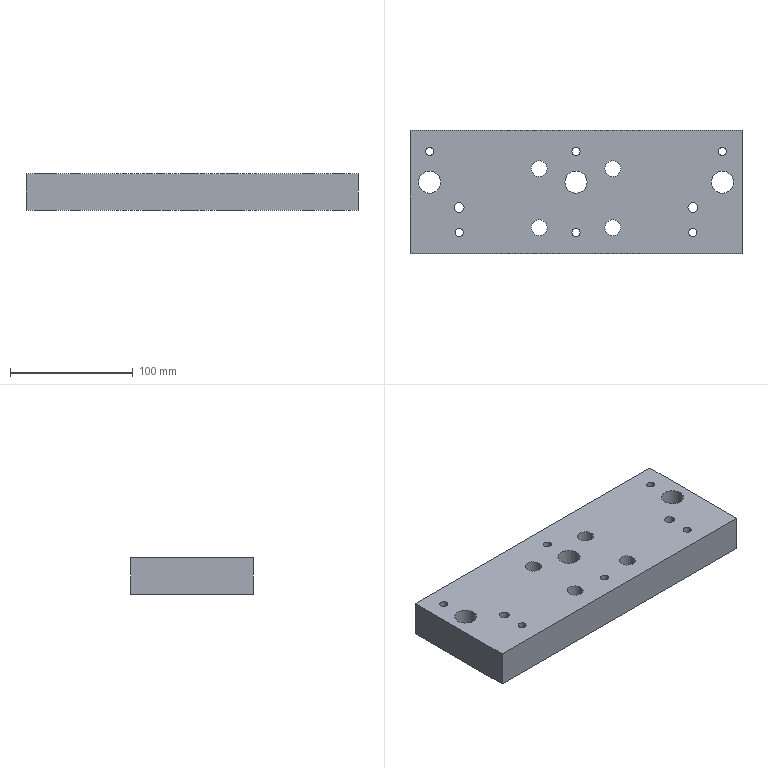Part | STEP file | TAM DE CHAY | 1 solid | 48 faces | box 270 x 100 x 30 mm | volume 752474 mm3 | cylinder 38 | plane 10 | commonest cylinder face diameters 6.647 x12 13 x8 20 x8 18 x6 8 x4